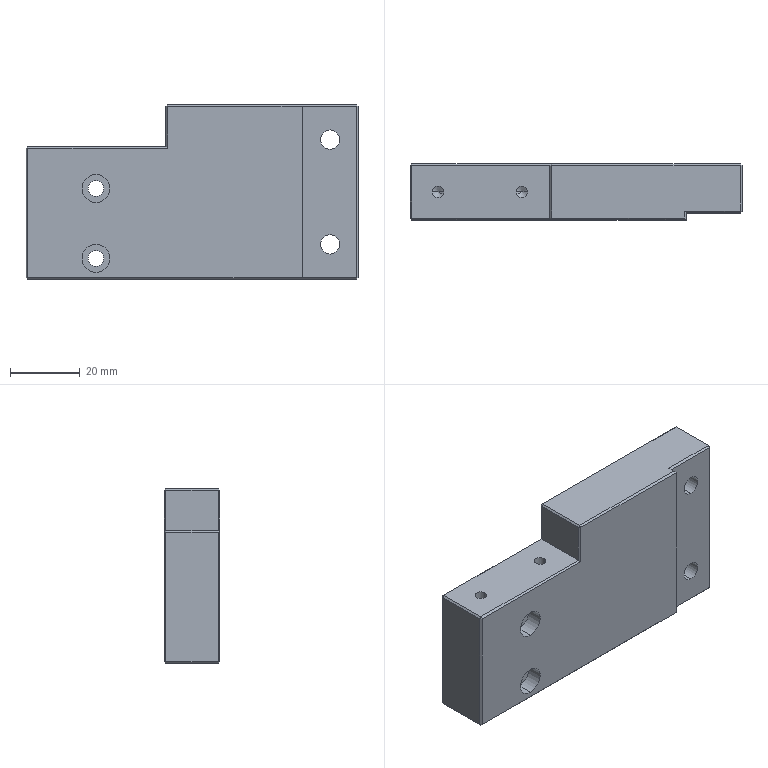Part | STEP file | ND25021-01-JDKM-28-TL | 1 solid | 69 faces | box 95 x 16 x 50 mm | volume 64378 mm3 | plane 45 | cylinder 20 | cone 4 | commonest cylinder face diameters 3.3 x4 4.5 x4 5.5 x4 8 x4 10 x4